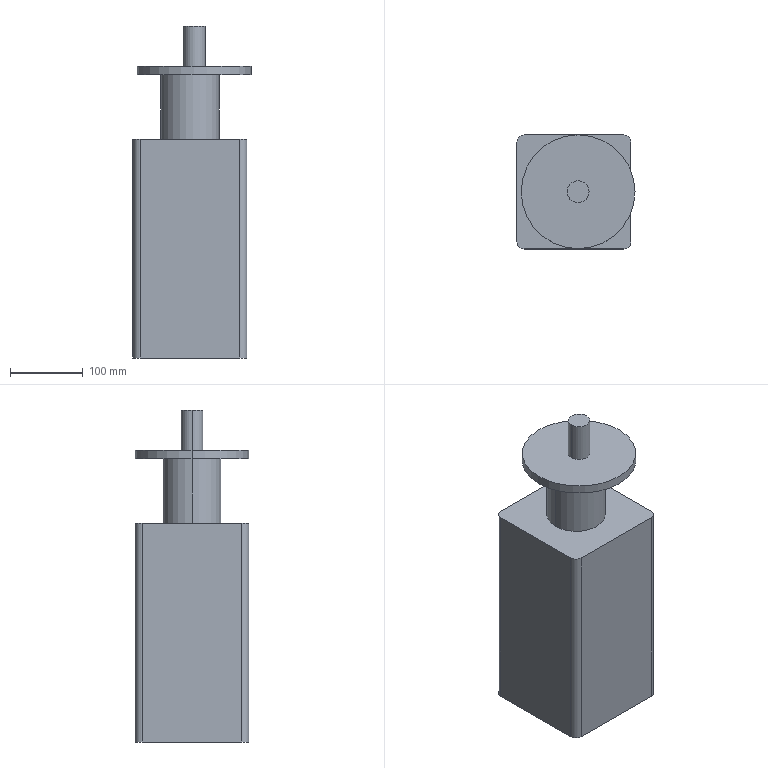Part | SolidWorks | features ICE 3, Extrusion 1, Fillet 1 | 1 solid | 19 faces | box 161.788 x 156 x 455 mm | volume 7985623 mm3 | cylinder 10 | plane 9 | commonest cylinder face diameters 20 x4 30 x2 80 x2 156 x2
STEP:
#1=CARTESIAN_POINT('',(98.788,78.,455.));
#2=VERTEX_POINT('',#1);
#3=CARTESIAN_POINT('',(68.788,78.,455.));
#4=VERTEX_POINT('',#3);
#5=CARTESIAN_POINT('',(83.788,78.,455.));
#6=DIRECTION('',(0.,0.,1.));
#7=DIRECTION('',(1.,0.,0.));
#8=AXIS2_PLACEMENT_3D('',#5,#6,#7);
#9=CIRCLE('',#8,15.);
#10=EDGE_CURVE('',#2,#4,#9,.T.);
#11=ORIENTED_EDGE('',*,*,#10,.F.);
#12=CARTESIAN_POINT('',(98.788,78.,400.));
#13=VERTEX_POINT('',#12);
#14=CARTESIAN_POINT('',(98.788,78.,455.));
#15=DIRECTION('',(0.,0.,-1.));
#16=VECTOR('',#15,1000.);
#17=LINE('',#14,#16);
#18=EDGE_CURVE('',#2,#13,#17,.T.);
#19=ORIENTED_EDGE('',*,*,#18,.T.);
#20=CARTESIAN_POINT('',(68.788,78.,400.));
#21=VERTEX_POINT('',#20);
#22=CARTESIAN_POINT('',(83.788,78.,400.));
#23=DIRECTION('',(0.,0.,1.));
#24=DIRECTION('',(1.,0.,0.));
#25=AXIS2_PLACEMENT_3D('',#22,#23,#24);
#26=CIRCLE('',#25,15.);
#27=EDGE_CURVE('',#13,#21,#26,.T.);
#28=ORIENTED_EDGE('',*,*,#27,.T.);
#29=CARTESIAN_POINT('',(68.788,78.,455.));
#30=DIRECTION('',(0.,0.,-1.));
#31=VECTOR('',#30,1000.);
#32=LINE('',#29,#31);
#33=EDGE_CURVE('',#4,#21,#32,.T.);
#34=ORIENTED_EDGE('',*,*,#33,.F.);
#35=EDGE_LOOP('',(#11,#19,#28,#34));
#36=FACE_OUTER_BOUND('',#35,.T.);
#37=CARTESIAN_POINT('',(83.788,78.,455.));
#38=DIRECTION('',(0.,0.,-1.));
#39=DIRECTION('',(-1.,0.,0.));
#40=AXIS2_PLACEMENT_3D('',#37,#38,#39);
#41=CYLINDRICAL_SURFACE('',#40,15.);
#42=ADVANCED_FACE('',(#36),#41,.T.);
#43=CARTESIAN_POINT('',(161.788,78.,400.));
#44=VERTEX_POINT('',#43);
#45=CARTESIAN_POINT('',(5.788,78.,400.));
#46=VERTEX_POINT('',#45);
#47=CARTESIAN_POINT('',(83.788,78.,400.));
#48=DIRECTION('',(0.,0.,1.));
#49=DIRECTION('',(1.,0.,0.));
#50=AXIS2_PLACEMENT_3D('',#47,#48,#49);
#51=CIRCLE('',#50,78.);
#52=EDGE_CURVE('',#44,#46,#51,.T.);
#53=ORIENTED_EDGE('',*,*,#52,.F.);
#54=CARTESIAN_POINT('',(161.788,78.,388.));
#55=VERTEX_POINT('',#54);
#56=CARTESIAN_POINT('',(161.788,78.,400.));
#57=DIRECTION('',(0.,0.,-1.));
#58=VECTOR('',#57,1000.);
#59=LINE('',#56,#58);
#60=EDGE_CURVE('',#44,#55,#59,.T.);
#61=ORIENTED_EDGE('',*,*,#60,.T.);
#62=CARTESIAN_POINT('',(5.788,78.,388.));
#63=VERTEX_POINT('',#62);
#64=CARTESIAN_POINT('',(83.788,78.,388.));
#65=DIRECTION('',(0.,0.,1.));
#66=DIRECTION('',(1.,0.,0.));
#67=AXIS2_PLACEMENT_3D('',#64,#65,#66);
#68=CIRCLE('',#67,78.);
#69=EDGE_CURVE('',#55,#63,#68,.T.);
#70=ORIENTED_EDGE('',*,*,#69,.T.);
#71=CARTESIAN_POINT('',(5.788,78.,400.));
#72=DIRECTION('',(0.,0.,-1.));
#73=VECTOR('',#72,1000.);
#74=LINE('',#71,#73);
#75=EDGE_CURVE('',#46,#63,#74,.T.);
#76=ORIENTED_EDGE('',*,*,#75,.F.);
#77=EDGE_LOOP('',(#53,#61,#70,#76));
#78=FACE_OUTER_BOUND('',#77,.T.);
#79=CARTESIAN_POINT('',(83.788,78.,400.));
#80=DIRECTION('',(0.,0.,-1.));
#81=DIRECTION('',(-1.,0.,0.));
#82=AXIS2_PLACEMENT_3D('',#79,#80,#81);
#83=CYLINDRICAL_SURFACE('',#82,78.);
#84=ADVANCED_FACE('',(#78),#83,.T.);
#85=CARTESIAN_POINT('',(118.,78.,388.));
#86=VERTEX_POINT('',#85);
#87=CARTESIAN_POINT('',(38.,78.,388.));
#88=VERTEX_POINT('',#87);
#89=CARTESIAN_POINT('',(78.,78.,388.));
#90=DIRECTION('',(0.,0.,1.));
#91=DIRECTION('',(1.,0.,0.));
#92=AXIS2_PLACEMENT_3D('',#89,#90,#91);
#93=CIRCLE('',#92,40.);
#94=EDGE_CURVE('',#86,#88,#93,.T.);
#95=ORIENTED_EDGE('',*,*,#94,.F.);
#96=CARTESIAN_POINT('',(118.,78.,300.));
#97=VERTEX_POINT('',#96);
#98=CARTESIAN_POINT('',(118.,78.,388.));
#99=DIRECTION('',(0.,0.,-1.));
#100=VECTOR('',#99,1000.);
#101=LINE('',#98,#100);
#102=EDGE_CURVE('',#86,#97,#101,.T.);
#103=ORIENTED_EDGE('',*,*,#102,.T.);
#104=CARTESIAN_POINT('',(38.,78.,300.));
#105=VERTEX_POINT('',#104);
#106=CARTESIAN_POINT('',(78.,78.,300.));
#107=DIRECTION('',(0.,0.,1.));
#108=DIRECTION('',(-1.,0.,0.));
#109=AXIS2_PLACEMENT_3D('',#106,#107,#108);
#110=CIRCLE('',#109,40.);
#111=EDGE_CURVE('',#97,#105,#110,.T.);
#112=ORIENTED_EDGE('',*,*,#111,.T.);
#113=CARTESIAN_POINT('',(38.,78.,388.));
#114=DIRECTION('',(0.,0.,-1.));
#115=VECTOR('',#114,1000.);
#116=LINE('',#113,#115);
#117=EDGE_CURVE('',#88,#105,#116,.T.);
#118=ORIENTED_EDGE('',*,*,#117,.F.);
#119=EDGE_LOOP('',(#95,#103,#112,#118));
#120=FACE_OUTER_BOUND('',#119,.T.);
#121=CARTESIAN_POINT('',(78.,78.,388.));
#122=DIRECTION('',(0.,0.,-1.));
#123=DIRECTION('',(-1.,0.,0.));
#124=AXIS2_PLACEMENT_3D('',#121,#122,#123);
#125=CYLINDRICAL_SURFACE('',#124,40.);
#126=ADVANCED_FACE('',(#120),#125,.T.);
#127=CARTESIAN_POINT('',(0.,146.,0.));
#128=VERTEX_POINT('',#127);
#129=CARTESIAN_POINT('',(0.,10.,0.));
#130=VERTEX_POINT('',#129);
#131=CARTESIAN_POINT('',(0.,0.,0.));
#132=DIRECTION('',(0.,-1.,0.));
#133=VECTOR('',#132,1000.);
#134=LINE('',#131,#133);
#135=EDGE_CURVE('',#128,#130,#134,.T.);
#136=ORIENTED_EDGE('',*,*,#135,.T.);
#137=CARTESIAN_POINT('',(0.,10.,300.));
#138=VERTEX_POINT('',#137);
#139=CARTESIAN_POINT('',(0.,10.,300.));
#140=DIRECTION('',(0.,0.,1.));
#141=VECTOR('',#140,1000.);
#142=LINE('',#139,#141);
#143=EDGE_CURVE('',#130,#138,#142,.T.);
#144=ORIENTED_EDGE('',*,*,#143,.T.);
#145=CARTESIAN_POINT('',(0.,146.,300.));
#146=VERTEX_POINT('',#145);
#147=CARTESIAN_POINT('',(0.,0.,300.));
#148=DIRECTION('',(0.,-1.,0.));
#149=VECTOR('',#148,1000.);
#150=LINE('',#147,#149);
#151=EDGE_CURVE('',#146,#138,#150,.T.);
#152=ORIENTED_EDGE('',*,*,#151,.F.);
#153=CARTESIAN_POINT('',(0.,146.,300.));
#154=DIRECTION('',(0.,0.,-1.));
#155=VECTOR('',#154,1000.);
#156=LINE('',#153,#155);
#157=EDGE_CURVE('',#146,#128,#156,.T.);
#158=ORIENTED_EDGE('',*,*,#157,.T.);
#159=EDGE_LOOP('',(#136,#144,#152,#158));
#160=FACE_OUTER_BOUND('',#159,.T.);
#161=CARTESIAN_POINT('',(0.,0.,300.));
#162=DIRECTION('',(1.,0.,0.));
#163=DIRECTION('',(0.,0.,-1.));
#164=AXIS2_PLACEMENT_3D('',#161,#162,#163);
#165=PLANE('',#164);
#166=ADVANCED_FACE('',(#160),#165,.F.);
#167=CARTESIAN_POINT('',(10.,0.,0.));
#168=VERTEX_POINT('',#167);
#169=CARTESIAN_POINT('',(146.,0.,0.));
#170=VERTEX_POINT('',#169);
#171=CARTESIAN_POINT('',(0.,0.,0.));
#172=DIRECTION('',(1.,0.,0.));
#173=VECTOR('',#172,1000.);
#174=LINE('',#171,#173);
#175=EDGE_CURVE('',#168,#170,#174,.T.);
#176=ORIENTED_EDGE('',*,*,#175,.T.);
#177=CARTESIAN_POINT('',(146.,0.,300.));
#178=VERTEX_POINT('',#177);
#179=CARTESIAN_POINT('',(146.,0.,300.));
#180=DIRECTION('',(0.,0.,1.));
#181=VECTOR('',#180,1000.);
#182=LINE('',#179,#181);
#183=EDGE_CURVE('',#170,#178,#182,.T.);
#184=ORIENTED_EDGE('',*,*,#183,.T.);
#185=CARTESIAN_POINT('',(10.,0.,300.));
#186=VERTEX_POINT('',#185);
#187=CARTESIAN_POINT('',(0.,0.,300.));
#188=DIRECTION('',(1.,0.,0.));
#189=VECTOR('',#188,1000.);
#190=LINE('',#187,#189);
#191=EDGE_CURVE('',#186,#178,#190,.T.);
#192=ORIENTED_EDGE('',*,*,#191,.F.);
#193=CARTESIAN_POINT('',(10.,0.,300.));
#194=DIRECTION('',(0.,0.,-1.));
#195=VECTOR('',#194,1000.);
#196=LINE('',#193,#195);
#197=EDGE_CURVE('',#186,#168,#196,.T.);
#198=ORIENTED_EDGE('',*,*,#197,.T.);
#199=EDGE_LOOP('',(#176,#184,#192,#198));
#200=FACE_OUTER_BOUND('',#199,.T.);
#201=CARTESIAN_POINT('',(0.,0.,300.));
#202=DIRECTION('',(0.,1.,0.));
#203=DIRECTION('',(0.,0.,1.));
#204=AXIS2_PLACEMENT_3D('',#201,#202,#203);
#205=PLANE('',#204);
#206=ADVANCED_FACE('',(#200),#205,.F.);
#207=CARTESIAN_POINT('',(156.,10.,300.));
#208=VERTEX_POINT('',#207);
#209=CARTESIAN_POINT('',(156.,146.,300.));
#210=VERTEX_POINT('',#209);
#211=CARTESIAN_POINT('',(156.,0.,300.));
#212=DIRECTION('',(0.,1.,0.));
#213=VECTOR('',#212,1000.);
#214=LINE('',#211,#213);
#215=EDGE_CURVE('',#208,#210,#214,.T.);
#216=ORIENTED_EDGE('',*,*,#215,.F.);
#217=CARTESIAN_POINT('',(156.,10.,0.));
#218=VERTEX_POINT('',#217);
#219=CARTESIAN_POINT('',(156.,10.,300.));
#220=DIRECTION('',(0.,0.,-1.));
#221=VECTOR('',#220,1000.);
#222=LINE('',#219,#221);
#223=EDGE_CURVE('',#208,#218,#222,.T.);
#224=ORIENTED_EDGE('',*,*,#223,.T.);
#225=CARTESIAN_POINT('',(156.,146.,0.));
#226=VERTEX_POINT('',#225);
#227=CARTESIAN_POINT('',(156.,0.,0.));
#228=DIRECTION('',(0.,1.,0.));
#229=VECTOR('',#228,1000.);
#230=LINE('',#227,#229);
#231=EDGE_CURVE('',#218,#226,#230,.T.);
#232=ORIENTED_EDGE('',*,*,#231,.T.);
#233=CARTESIAN_POINT('',(156.,146.,300.));
#234=DIRECTION('',(0.,0.,1.));
#235=VECTOR('',#234,1000.);
#236=LINE('',#233,#235);
#237=EDGE_CURVE('',#226,#210,#236,.T.);
#238=ORIENTED_EDGE('',*,*,#237,.T.);
#239=EDGE_LOOP('',(#216,#224,#232,#238));
#240=FACE_OUTER_BOUND('',#239,.T.);
#241=CARTESIAN_POINT('',(156.,0.,300.));
#242=DIRECTION('',(-1.,0.,0.));
#243=DIRECTION('',(0.,-1.,0.));
#244=AXIS2_PLACEMENT_3D('',#241,#242,#243);
#245=PLANE('',#244);
#246=ADVANCED_FACE('',(#240),#245,.F.);
#247=CARTESIAN_POINT('',(146.,156.,300.));
#248=VERTEX_POINT('',#247);
#249=CARTESIAN_POINT('',(10.,156.,300.));
#250=VERTEX_POINT('',#249);
#251=CARTESIAN_POINT('',(0.,156.,300.));
#252=DIRECTION('',(-1.,0.,0.));
#253=VECTOR('',#252,1000.);
#254=LINE('',#251,#253);
#255=EDGE_CURVE('',#248,#250,#254,.T.);
#256=ORIENTED_EDGE('',*,*,#255,.F.);
#257=CARTESIAN_POINT('',(146.,156.,0.));
#258=VERTEX_POINT('',#257);
#259=CARTESIAN_POINT('',(146.,156.,300.));
#260=DIRECTION('',(0.,0.,-1.));
#261=VECTOR('',#260,1000.);
#262=LINE('',#259,#261);
#263=EDGE_CURVE('',#248,#258,#262,.T.);
#264=ORIENTED_EDGE('',*,*,#263,.T.);
#265=CARTESIAN_POINT('',(10.,156.,0.));
#266=VERTEX_POINT('',#265);
#267=CARTESIAN_POINT('',(0.,156.,0.));
#268=DIRECTION('',(-1.,0.,0.));
#269=VECTOR('',#268,1000.);
#270=LINE('',#267,#269);
#271=EDGE_CURVE('',#258,#266,#270,.T.);
#272=ORIENTED_EDGE('',*,*,#271,.T.);
#273=CARTESIAN_POINT('',(10.,156.,300.));
#274=DIRECTION('',(0.,0.,1.));
#275=VECTOR('',#274,1000.);
#276=LINE('',#273,#275);
#277=EDGE_CURVE('',#266,#250,#276,.T.);
#278=ORIENTED_EDGE('',*,*,#277,.T.);
#279=EDGE_LOOP('',(#256,#264,#272,#278));
#280=FACE_OUTER_BOUND('',#279,.T.);
#281=CARTESIAN_POINT('',(0.,156.,300.));
#282=DIRECTION('',(0.,-1.,0.));
#283=DIRECTION('',(0.,0.,-1.));
#284=AXIS2_PLACEMENT_3D('',#281,#282,#283);
#285=PLANE('',#284);
#286=ADVANCED_FACE('',(#280),#285,.F.);
#287=CARTESIAN_POINT('',(78.,78.,300.));
#288=DIRECTION('',(0.,0.,1.));
#289=DIRECTION('',(-1.,0.,0.));
#290=AXIS2_PLACEMENT_3D('',#287,#288,#289);
#291=CIRCLE('',#290,40.);
#292=EDGE_CURVE('',#105,#97,#291,.T.);
#293=ORIENTED_EDGE('',*,*,#292,.F.);
#294=ORIENTED_EDGE('',*,*,#111,.F.);
#295=EDGE_LOOP('',(#293,#294));
#296=FACE_BOUND('',#295,.T.);
#297=ORIENTED_EDGE('',*,*,#191,.T.);
#298=CARTESIAN_POINT('',(146.,10.,300.));
#299=DIRECTION('',(0.,0.,1.));
#300=DIRECTION('',(-1.,0.,0.));
#301=AXIS2_PLACEMENT_3D('',#298,#299,#300);
#302=CIRCLE('',#301,10.);
#303=EDGE_CURVE('',#178,#208,#302,.T.);
#304=ORIENTED_EDGE('',*,*,#303,.T.);
#305=ORIENTED_EDGE('',*,*,#215,.T.);
#306=CARTESIAN_POINT('',(146.,146.,300.));
#307=DIRECTION('',(0.,0.,1.));
#308=DIRECTION('',(-1.,0.,0.));
#309=AXIS2_PLACEMENT_3D('',#306,#307,#308);
#310=CIRCLE('',#309,10.);
#311=EDGE_CURVE('',#210,#248,#310,.T.);
#312=ORIENTED_EDGE('',*,*,#311,.T.);
#313=ORIENTED_EDGE('',*,*,#255,.T.);
#314=CARTESIAN_POINT('',(10.,146.,300.));
#315=DIRECTION('',(0.,0.,1.));
#316=DIRECTION('',(-1.,0.,0.));
#317=AXIS2_PLACEMENT_3D('',#314,#315,#316);
#318=CIRCLE('',#317,10.);
#319=EDGE_CURVE('',#250,#146,#318,.T.);
#320=ORIENTED_EDGE('',*,*,#319,.T.);
#321=ORIENTED_EDGE('',*,*,#151,.T.);
#322=CARTESIAN_POINT('',(10.,10.,300.));
#323=DIRECTION('',(0.,0.,1.));
#324=DIRECTION('',(-1.,0.,0.));
#325=AXIS2_PLACEMENT_3D('',#322,#323,#324);
#326=CIRCLE('',#325,10.);
#327=EDGE_CURVE('',#138,#186,#326,.T.);
#328=ORIENTED_EDGE('',*,*,#327,.T.);
#329=EDGE_LOOP('',(#297,#304,#305,#312,#313,#320,#321,#328));
#330=FACE_OUTER_BOUND('',#329,.T.);
#331=CARTESIAN_POINT('',(0.,0.,300.));
#332=DIRECTION('',(0.,0.,-1.));
#333=DIRECTION('',(-1.,0.,0.));
#334=AXIS2_PLACEMENT_3D('',#331,#332,#333);
#335=PLANE('',#334);
#336=ADVANCED_FACE('',(#296,#330),#335,.F.);
#337=ORIENTED_EDGE('',*,*,#231,.F.);
#338=CARTESIAN_POINT('',(146.,10.,0.));
#339=DIRECTION('',(0.,0.,-1.));
#340=DIRECTION('',(-1.,0.,0.));
#341=AXIS2_PLACEMENT_3D('',#338,#339,#340);
#342=CIRCLE('',#341,10.);
#343=EDGE_CURVE('',#218,#170,#342,.T.);
#344=ORIENTED_EDGE('',*,*,#343,.T.);
#345=ORIENTED_EDGE('',*,*,#175,.F.);
#346=CARTESIAN_POINT('',(10.,10.,0.));
#347=DIRECTION('',(0.,0.,-1.));
#348=DIRECTION('',(-1.,0.,0.));
#349=AXIS2_PLACEMENT_3D('',#346,#347,#348);
#350=CIRCLE('',#349,10.);
#351=EDGE_CURVE('',#168,#130,#350,.T.);
#352=ORIENTED_EDGE('',*,*,#351,.T.);
#353=ORIENTED_EDGE('',*,*,#135,.F.);
#354=CARTESIAN_POINT('',(10.,146.,0.));
#355=DIRECTION('',(0.,0.,-1.));
#356=DIRECTION('',(-1.,0.,0.));
#357=AXIS2_PLACEMENT_3D('',#354,#355,#356);
#358=CIRCLE('',#357,10.);
#359=EDGE_CURVE('',#128,#266,#358,.T.);
#360=ORIENTED_EDGE('',*,*,#359,.T.);
#361=ORIENTED_EDGE('',*,*,#271,.F.);
#362=CARTESIAN_POINT('',(146.,146.,0.));
#363=DIRECTION('',(0.,0.,-1.));
#364=DIRECTION('',(-1.,0.,0.));
#365=AXIS2_PLACEMENT_3D('',#362,#363,#364);
#366=CIRCLE('',#365,10.);
#367=EDGE_CURVE('',#258,#226,#366,.T.);
#368=ORIENTED_EDGE('',*,*,#367,.T.);
#369=EDGE_LOOP('',(#337,#344,#345,#352,#353,#360,#361,#368));
#370=FACE_OUTER_BOUND('',#369,.T.);
#371=CARTESIAN_POINT('',(0.,0.,0.));
#372=DIRECTION('',(0.,0.,-1.));
#373=DIRECTION('',(-1.,0.,0.));
#374=AXIS2_PLACEMENT_3D('',#371,#372,#373);
#375=PLANE('',#374);
#376=ADVANCED_FACE('',(#370),#375,.T.);
#377=ORIENTED_EDGE('',*,*,#102,.F.);
#378=CARTESIAN_POINT('',(78.,78.,388.));
#379=DIRECTION('',(0.,0.,1.));
#380=DIRECTION('',(1.,0.,0.));
#381=AXIS2_PLACEMENT_3D('',#378,#379,#380);
#382=CIRCLE('',#381,40.);
#383=EDGE_CURVE('',#88,#86,#382,.T.);
#384=ORIENTED_EDGE('',*,*,#383,.F.);
#385=ORIENTED_EDGE('',*,*,#117,.T.);
#386=ORIENTED_EDGE('',*,*,#292,.T.);
#387=EDGE_LOOP('',(#377,#384,#385,#386));
#388=FACE_OUTER_BOUND('',#387,.T.);
#389=CARTESIAN_POINT('',(78.,78.,388.));
#390=DIRECTION('',(0.,0.,-1.));
#391=DIRECTION('',(-1.,0.,0.));
#392=AXIS2_PLACEMENT_3D('',#389,#390,#391);
#393=CYLINDRICAL_SURFACE('',#392,40.);
#394=ADVANCED_FACE('',(#388),#393,.T.);
#395=ORIENTED_EDGE('',*,*,#60,.F.);
#396=CARTESIAN_POINT('',(83.788,78.,400.));
#397=DIRECTION('',(0.,0.,1.));
#398=DIRECTION('',(1.,0.,0.));
#399=AXIS2_PLACEMENT_3D('',#396,#397,#398);
#400=CIRCLE('',#399,78.);
#401=EDGE_CURVE('',#46,#44,#400,.T.);
#402=ORIENTED_EDGE('',*,*,#401,.F.);
#403=ORIENTED_EDGE('',*,*,#75,.T.);
#404=CARTESIAN_POINT('',(83.788,78.,388.));
#405=DIRECTION('',(0.,0.,1.));
#406=DIRECTION('',(1.,0.,0.));
#407=AXIS2_PLACEMENT_3D('',#404,#405,#406);
#408=CIRCLE('',#407,78.);
#409=EDGE_CURVE('',#63,#55,#408,.T.);
#410=ORIENTED_EDGE('',*,*,#409,.T.);
#411=EDGE_LOOP('',(#395,#402,#403,#410));
#412=FACE_OUTER_BOUND('',#411,.T.);
#413=CARTESIAN_POINT('',(83.788,78.,400.));
#414=DIRECTION('',(0.,0.,-1.));
#415=DIRECTION('',(-1.,0.,0.));
#416=AXIS2_PLACEMENT_3D('',#413,#414,#415);
#417=CYLINDRICAL_SURFACE('',#416,78.);
#418=ADVANCED_FACE('',(#412),#417,.T.);
#419=CARTESIAN_POINT('',(83.788,78.,400.));
#420=DIRECTION('',(0.,0.,1.));
#421=DIRECTION('',(1.,0.,0.));
#422=AXIS2_PLACEMENT_3D('',#419,#420,#421);
#423=CIRCLE('',#422,15.);
#424=EDGE_CURVE('',#21,#13,#423,.T.);
#425=ORIENTED_EDGE('',*,*,#424,.F.);
#426=ORIENTED_EDGE('',*,*,#27,.F.);
#427=EDGE_LOOP('',(#425,#426));
#428=FACE_BOUND('',#427,.T.);
#429=ORIENTED_EDGE('',*,*,#401,.T.);
#430=ORIENTED_EDGE('',*,*,#52,.T.);
#431=EDGE_LOOP('',(#429,#430));
#432=FACE_OUTER_BOUND('',#431,.T.);
#433=CARTESIAN_POINT('',(83.788,78.,400.));
#434=DIRECTION('',(0.,0.,1.));
#435=DIRECTION('',(1.,0.,0.));
#436=AXIS2_PLACEMENT_3D('',#433,#434,#435);
#437=PLANE('',#436);
#438=ADVANCED_FACE('',(#428,#432),#437,.T.);
#439=ORIENTED_EDGE('',*,*,#383,.T.);
#440=ORIENTED_EDGE('',*,*,#94,.T.);
#441=EDGE_LOOP('',(#439,#440));
#442=FACE_BOUND('',#441,.T.);
#443=ORIENTED_EDGE('',*,*,#409,.F.);
#444=ORIENTED_EDGE('',*,*,#69,.F.);
#445=EDGE_LOOP('',(#443,#444));
#446=FACE_OUTER_BOUND('',#445,.T.);
#447=CARTESIAN_POINT('',(83.788,78.,388.));
#448=DIRECTION('',(0.,0.,1.));
#449=DIRECTION('',(1.,0.,0.));
#450=AXIS2_PLACEMENT_3D('',#447,#448,#449);
#451=PLANE('',#450);
#452=ADVANCED_FACE('',(#442,#446),#451,.F.);
#453=ORIENTED_EDGE('',*,*,#303,.F.);
#454=ORIENTED_EDGE('',*,*,#183,.F.);
#455=ORIENTED_EDGE('',*,*,#343,.F.);
#456=ORIENTED_EDGE('',*,*,#223,.F.);
#457=EDGE_LOOP('',(#453,#454,#455,#456));
#458=FACE_OUTER_BOUND('',#457,.T.);
#459=CARTESIAN_POINT('',(146.,10.,300.));
#460=DIRECTION('',(0.,0.,-1.));
#461=DIRECTION('',(-1.,0.,0.));
#462=AXIS2_PLACEMENT_3D('',#459,#460,#461);
#463=CYLINDRICAL_SURFACE('',#462,10.);
#464=ADVANCED_FACE('',(#458),#463,.T.);
#465=ORIENTED_EDGE('',*,*,#327,.F.);
#466=ORIENTED_EDGE('',*,*,#143,.F.);
#467=ORIENTED_EDGE('',*,*,#351,.F.);
#468=ORIENTED_EDGE('',*,*,#197,.F.);
#469=EDGE_LOOP('',(#465,#466,#467,#468));
#470=FACE_OUTER_BOUND('',#469,.T.);
#471=CARTESIAN_POINT('',(10.,10.,300.));
#472=DIRECTION('',(0.,0.,-1.));
#473=DIRECTION('',(-1.,0.,0.));
#474=AXIS2_PLACEMENT_3D('',#471,#472,#473);
#475=CYLINDRICAL_SURFACE('',#474,10.);
#476=ADVANCED_FACE('',(#470),#475,.T.);
#477=ORIENTED_EDGE('',*,*,#311,.F.);
#478=ORIENTED_EDGE('',*,*,#237,.F.);
#479=ORIENTED_EDGE('',*,*,#367,.F.);
#480=ORIENTED_EDGE('',*,*,#263,.F.);
#481=EDGE_LOOP('',(#477,#478,#479,#480));
#482=FACE_OUTER_BOUND('',#481,.T.);
#483=CARTESIAN_POINT('',(146.,146.,300.));
#484=DIRECTION('',(0.,0.,-1.));
#485=DIRECTION('',(-1.,0.,0.));
#486=AXIS2_PLACEMENT_3D('',#483,#484,#485);
#487=CYLINDRICAL_SURFACE('',#486,10.);
#488=ADVANCED_FACE('',(#482),#487,.T.);
#489=ORIENTED_EDGE('',*,*,#319,.F.);
#490=ORIENTED_EDGE('',*,*,#277,.F.);
#491=ORIENTED_EDGE('',*,*,#359,.F.);
#492=ORIENTED_EDGE('',*,*,#157,.F.);
#493=EDGE_LOOP('',(#489,#490,#491,#492));
#494=FACE_OUTER_BOUND('',#493,.T.);
#495=CARTESIAN_POINT('',(10.,146.,300.));
#496=DIRECTION('',(0.,0.,-1.));
#497=DIRECTION('',(-1.,0.,0.));
#498=AXIS2_PLACEMENT_3D('',#495,#496,#497);
#499=CYLINDRICAL_SURFACE('',#498,10.);
#500=ADVANCED_FACE('',(#494),#499,.T.);
#501=ORIENTED_EDGE('',*,*,#18,.F.);
#502=CARTESIAN_POINT('',(83.788,78.,455.));
#503=DIRECTION('',(0.,0.,1.));
#504=DIRECTION('',(1.,0.,0.));
#505=AXIS2_PLACEMENT_3D('',#502,#503,#504);
#506=CIRCLE('',#505,15.);
#507=EDGE_CURVE('',#4,#2,#506,.T.);
#508=ORIENTED_EDGE('',*,*,#507,.F.);
#509=ORIENTED_EDGE('',*,*,#33,.T.);
#510=ORIENTED_EDGE('',*,*,#424,.T.);
#511=EDGE_LOOP('',(#501,#508,#509,#510));
#512=FACE_OUTER_BOUND('',#511,.T.);
#513=CARTESIAN_POINT('',(83.788,78.,455.));
#514=DIRECTION('',(0.,0.,-1.));
#515=DIRECTION('',(-1.,0.,0.));
#516=AXIS2_PLACEMENT_3D('',#513,#514,#515);
#517=CYLINDRICAL_SURFACE('',#516,15.);
#518=ADVANCED_FACE('',(#512),#517,.T.);
#519=ORIENTED_EDGE('',*,*,#507,.T.);
#520=ORIENTED_EDGE('',*,*,#10,.T.);
#521=EDGE_LOOP('',(#519,#520));
#522=FACE_OUTER_BOUND('',#521,.T.);
#523=CARTESIAN_POINT('',(83.788,78.,455.));
#524=DIRECTION('',(0.,0.,1.));
#525=DIRECTION('',(1.,0.,0.));
#526=AXIS2_PLACEMENT_3D('',#523,#524,#525);
#527=PLANE('',#526);
#528=ADVANCED_FACE('',(#522),#527,.T.);
#529=CLOSED_SHELL('',(#42,#84,#126,#166,#206,#246,#286,#336,#376,#394,#418,#438,#452,#464,#476,#488,#500,#518,#528));
#530=MANIFOLD_SOLID_BREP('',#529);
#531=CARTESIAN_POINT('',(0.,0.,0.));
#532=DIRECTION('',(0.,0.,1.));
#533=DIRECTION('',(1.,0.,0.));
#534=AXIS2_PLACEMENT_3D('',#531,#532,#533);
#535=(LENGTH_UNIT()NAMED_UNIT(*)SI_UNIT(.MILLI.,.METRE.));
#536=UNCERTAINTY_MEASURE_WITH_UNIT(LENGTH_MEASURE(0.00001),#535,'','');
#537=(NAMED_UNIT(*)PLANE_ANGLE_UNIT()SI_UNIT($,.RADIAN.));
#538=(NAMED_UNIT(*)SI_UNIT($,.STERADIAN.)SOLID_ANGLE_UNIT());
#539=(GEOMETRIC_REPRESENTATION_CONTEXT(3)GLOBAL_UNCERTAINTY_ASSIGNED_CONTEXT((#536))GLOBAL_UNIT_ASSIGNED_CONTEXT((#535,#537,#538))REPRESENTATION_CONTEXT('',''));
#540=ADVANCED_BREP_SHAPE_REPRESENTATION('',(#530,#534),#539);